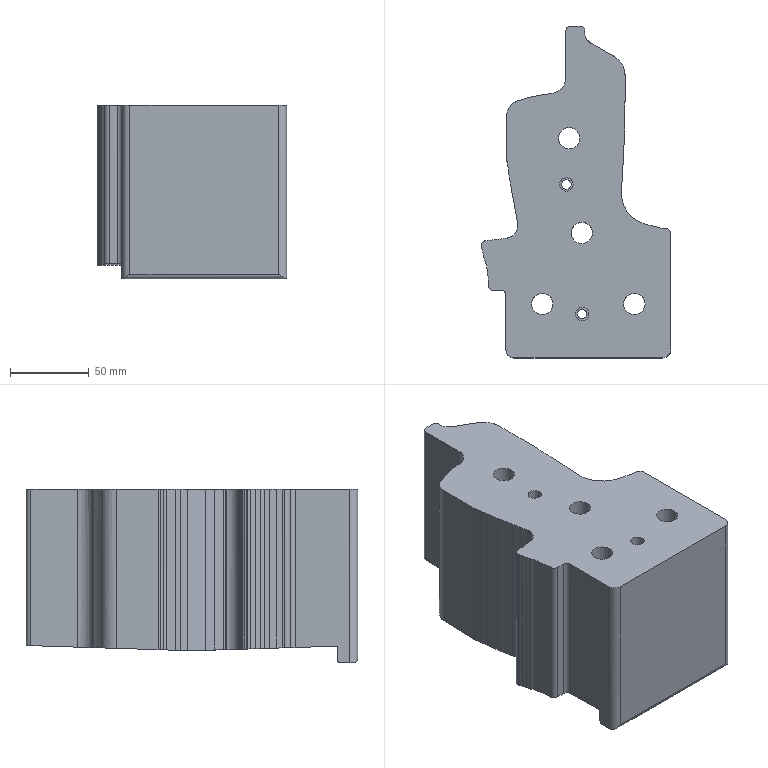Part | STEP file | lll_id262_x_t | 1 solid | 107 faces | box 119.869 x 210 x 110 mm | volume 1536822 mm3 | cylinder 82 | plane 23 | cone 2 | commonest cylinder face diameters 6 x10 13.509 x4 20.007 x4 8.5 x2 10 x2 10.505 x2